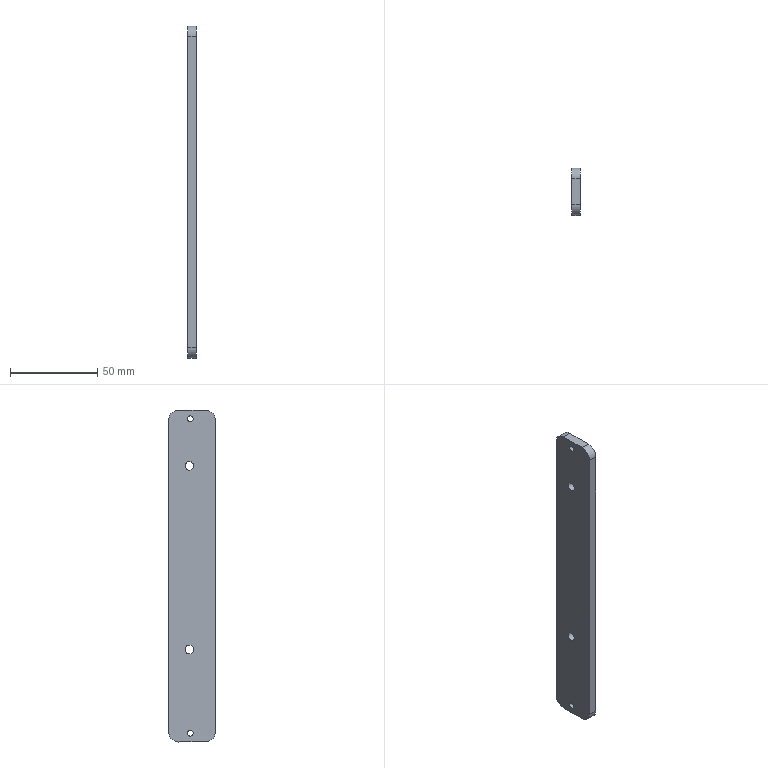Part | NX | 1 solid | 14 faces | box 5 x 27 x 190 mm | volume 25214 mm3 | cylinder 8 | plane 6 | commonest cylinder face diameters 12 x4 3.3 x2 5 x2
STEP:
#1=CARTESIAN_POINT('',(210.423,-113.198,-7.805));
#2=VERTEX_POINT('',#1);
#3=CARTESIAN_POINT('',(210.423,-113.198,170.195));
#4=VERTEX_POINT('',#3);
#5=CARTESIAN_POINT('',(210.423,-113.198,-13.805));
#6=DIRECTION('',(0.,0.,1.));
#7=VECTOR('',#6,1000.);
#8=LINE('',#5,#7);
#9=EDGE_CURVE('',#2,#4,#8,.T.);
#10=ORIENTED_EDGE('',*,*,#9,.F.);
#11=CARTESIAN_POINT('',(205.423,-113.198,-7.805));
#12=VERTEX_POINT('',#11);
#13=CARTESIAN_POINT('',(210.423,-113.198,-7.805));
#14=DIRECTION('',(-1.,0.,0.));
#15=VECTOR('',#14,1000.);
#16=LINE('',#13,#15);
#17=EDGE_CURVE('',#2,#12,#16,.T.);
#18=ORIENTED_EDGE('',*,*,#17,.T.);
#19=CARTESIAN_POINT('',(205.423,-113.198,170.195));
#20=VERTEX_POINT('',#19);
#21=CARTESIAN_POINT('',(205.423,-113.198,-13.805));
#22=DIRECTION('',(0.,0.,1.));
#23=VECTOR('',#22,1000.);
#24=LINE('',#21,#23);
#25=EDGE_CURVE('',#12,#20,#24,.T.);
#26=ORIENTED_EDGE('',*,*,#25,.T.);
#27=CARTESIAN_POINT('',(210.423,-113.198,170.195));
#28=DIRECTION('',(1.,0.,0.));
#29=VECTOR('',#28,1000.);
#30=LINE('',#27,#29);
#31=EDGE_CURVE('',#20,#4,#30,.T.);
#32=ORIENTED_EDGE('',*,*,#31,.T.);
#33=EDGE_LOOP('',(#10,#18,#26,#32));
#34=FACE_BOUND('',#33,.T.);
#35=CARTESIAN_POINT('',(210.423,-113.198,-13.805));
#36=DIRECTION('',(0.,-1.,0.));
#37=DIRECTION('',(-1.,0.,0.));
#38=AXIS2_PLACEMENT_3D('',#35,#36,#37);
#39=PLANE('',#38);
#40=ADVANCED_FACE('',(#34),#39,.F.);
#41=CARTESIAN_POINT('',(205.423,-119.198,176.195));
#42=VERTEX_POINT('',#41);
#43=CARTESIAN_POINT('',(205.423,-134.198,176.195));
#44=VERTEX_POINT('',#43);
#45=CARTESIAN_POINT('',(205.423,-140.198,176.195));
#46=DIRECTION('',(0.,-1.,0.));
#47=VECTOR('',#46,1000.);
#48=LINE('',#45,#47);
#49=EDGE_CURVE('',#42,#44,#48,.T.);
#50=ORIENTED_EDGE('',*,*,#49,.T.);
#51=CARTESIAN_POINT('',(210.423,-134.198,176.195));
#52=VERTEX_POINT('',#51);
#53=CARTESIAN_POINT('',(210.423,-134.198,176.195));
#54=DIRECTION('',(1.,0.,0.));
#55=VECTOR('',#54,1000.);
#56=LINE('',#53,#55);
#57=EDGE_CURVE('',#44,#52,#56,.T.);
#58=ORIENTED_EDGE('',*,*,#57,.T.);
#59=CARTESIAN_POINT('',(210.423,-119.198,176.195));
#60=VERTEX_POINT('',#59);
#61=CARTESIAN_POINT('',(210.423,-140.198,176.195));
#62=DIRECTION('',(0.,-1.,0.));
#63=VECTOR('',#62,1000.);
#64=LINE('',#61,#63);
#65=EDGE_CURVE('',#60,#52,#64,.T.);
#66=ORIENTED_EDGE('',*,*,#65,.F.);
#67=CARTESIAN_POINT('',(210.423,-119.198,176.195));
#68=DIRECTION('',(-1.,0.,0.));
#69=VECTOR('',#68,1000.);
#70=LINE('',#67,#69);
#71=EDGE_CURVE('',#60,#42,#70,.T.);
#72=ORIENTED_EDGE('',*,*,#71,.T.);
#73=EDGE_LOOP('',(#50,#58,#66,#72));
#74=FACE_BOUND('',#73,.T.);
#75=CARTESIAN_POINT('',(210.423,-140.198,176.195));
#76=DIRECTION('',(0.,0.,-1.));
#77=DIRECTION('',(0.,-1.,0.));
#78=AXIS2_PLACEMENT_3D('',#75,#76,#77);
#79=PLANE('',#78);
#80=ADVANCED_FACE('',(#74),#79,.F.);
#81=CARTESIAN_POINT('',(205.423,-140.198,170.195));
#82=VERTEX_POINT('',#81);
#83=CARTESIAN_POINT('',(205.423,-140.198,-7.805));
#84=VERTEX_POINT('',#83);
#85=CARTESIAN_POINT('',(205.423,-140.198,-13.805));
#86=DIRECTION('',(0.,0.,-1.));
#87=VECTOR('',#86,1000.);
#88=LINE('',#85,#87);
#89=EDGE_CURVE('',#82,#84,#88,.T.);
#90=ORIENTED_EDGE('',*,*,#89,.T.);
#91=CARTESIAN_POINT('',(210.423,-140.198,-7.805));
#92=VERTEX_POINT('',#91);
#93=CARTESIAN_POINT('',(210.423,-140.198,-7.805));
#94=DIRECTION('',(1.,0.,0.));
#95=VECTOR('',#94,1000.);
#96=LINE('',#93,#95);
#97=EDGE_CURVE('',#84,#92,#96,.T.);
#98=ORIENTED_EDGE('',*,*,#97,.T.);
#99=CARTESIAN_POINT('',(210.423,-140.198,170.195));
#100=VERTEX_POINT('',#99);
#101=CARTESIAN_POINT('',(210.423,-140.198,-13.805));
#102=DIRECTION('',(0.,0.,-1.));
#103=VECTOR('',#102,1000.);
#104=LINE('',#101,#103);
#105=EDGE_CURVE('',#100,#92,#104,.T.);
#106=ORIENTED_EDGE('',*,*,#105,.F.);
#107=CARTESIAN_POINT('',(210.423,-140.198,170.195));
#108=DIRECTION('',(-1.,0.,0.));
#109=VECTOR('',#108,1000.);
#110=LINE('',#107,#109);
#111=EDGE_CURVE('',#100,#82,#110,.T.);
#112=ORIENTED_EDGE('',*,*,#111,.T.);
#113=EDGE_LOOP('',(#90,#98,#106,#112));
#114=FACE_BOUND('',#113,.T.);
#115=CARTESIAN_POINT('',(210.423,-140.198,-13.805));
#116=DIRECTION('',(0.,1.,0.));
#117=DIRECTION('',(0.,0.,-1.));
#118=AXIS2_PLACEMENT_3D('',#115,#116,#117);
#119=PLANE('',#118);
#120=ADVANCED_FACE('',(#114),#119,.F.);
#121=CARTESIAN_POINT('',(205.423,-134.198,-13.805));
#122=VERTEX_POINT('',#121);
#123=CARTESIAN_POINT('',(205.423,-119.198,-13.805));
#124=VERTEX_POINT('',#123);
#125=CARTESIAN_POINT('',(205.423,-140.198,-13.805));
#126=DIRECTION('',(0.,1.,0.));
#127=VECTOR('',#126,1000.);
#128=LINE('',#125,#127);
#129=EDGE_CURVE('',#122,#124,#128,.T.);
#130=ORIENTED_EDGE('',*,*,#129,.T.);
#131=CARTESIAN_POINT('',(210.423,-119.198,-13.805));
#132=VERTEX_POINT('',#131);
#133=CARTESIAN_POINT('',(210.423,-119.198,-13.805));
#134=DIRECTION('',(1.,0.,0.));
#135=VECTOR('',#134,1000.);
#136=LINE('',#133,#135);
#137=EDGE_CURVE('',#124,#132,#136,.T.);
#138=ORIENTED_EDGE('',*,*,#137,.T.);
#139=CARTESIAN_POINT('',(210.423,-134.198,-13.805));
#140=VERTEX_POINT('',#139);
#141=CARTESIAN_POINT('',(210.423,-140.198,-13.805));
#142=DIRECTION('',(0.,1.,0.));
#143=VECTOR('',#142,1000.);
#144=LINE('',#141,#143);
#145=EDGE_CURVE('',#140,#132,#144,.T.);
#146=ORIENTED_EDGE('',*,*,#145,.F.);
#147=CARTESIAN_POINT('',(210.423,-134.198,-13.805));
#148=DIRECTION('',(-1.,0.,0.));
#149=VECTOR('',#148,1000.);
#150=LINE('',#147,#149);
#151=EDGE_CURVE('',#140,#122,#150,.T.);
#152=ORIENTED_EDGE('',*,*,#151,.T.);
#153=EDGE_LOOP('',(#130,#138,#146,#152));
#154=FACE_BOUND('',#153,.T.);
#155=CARTESIAN_POINT('',(210.423,-140.198,-13.805));
#156=DIRECTION('',(0.,0.,1.));
#157=DIRECTION('',(0.,-1.,0.));
#158=AXIS2_PLACEMENT_3D('',#155,#156,#157);
#159=PLANE('',#158);
#160=ADVANCED_FACE('',(#154),#159,.F.);
#161=CARTESIAN_POINT('',(210.423,-127.744,144.196));
#162=VERTEX_POINT('',#161);
#163=CARTESIAN_POINT('',(210.423,-125.244,144.196));
#164=DIRECTION('',(1.,0.,0.));
#165=DIRECTION('',(0.,-1.,0.));
#166=AXIS2_PLACEMENT_3D('',#163,#164,#165);
#167=CIRCLE('',#166,2.5);
#168=EDGE_CURVE('',#162,#162,#167,.T.);
#169=ORIENTED_EDGE('',*,*,#168,.F.);
#170=EDGE_LOOP('',(#169));
#171=FACE_BOUND('',#170,.T.);
#172=CARTESIAN_POINT('',(210.423,-127.744,39.152));
#173=VERTEX_POINT('',#172);
#174=CARTESIAN_POINT('',(210.423,-125.244,39.152));
#175=DIRECTION('',(1.,0.,0.));
#176=DIRECTION('',(0.,-1.,0.));
#177=AXIS2_PLACEMENT_3D('',#174,#175,#176);
#178=CIRCLE('',#177,2.5);
#179=EDGE_CURVE('',#173,#173,#178,.T.);
#180=ORIENTED_EDGE('',*,*,#179,.F.);
#181=EDGE_LOOP('',(#180));
#182=FACE_BOUND('',#181,.T.);
#183=CARTESIAN_POINT('',(210.423,-127.348,171.2));
#184=VERTEX_POINT('',#183);
#185=CARTESIAN_POINT('',(210.423,-125.698,171.2));
#186=DIRECTION('',(-1.,0.,0.));
#187=DIRECTION('',(0.,-1.,0.));
#188=AXIS2_PLACEMENT_3D('',#185,#186,#187);
#189=CIRCLE('',#188,1.65);
#190=EDGE_CURVE('',#184,#184,#189,.T.);
#191=ORIENTED_EDGE('',*,*,#190,.T.);
#192=EDGE_LOOP('',(#191));
#193=FACE_BOUND('',#192,.T.);
#194=CARTESIAN_POINT('',(210.423,-127.348,-8.8));
#195=VERTEX_POINT('',#194);
#196=CARTESIAN_POINT('',(210.423,-125.698,-8.8));
#197=DIRECTION('',(-1.,0.,0.));
#198=DIRECTION('',(0.,-1.,0.));
#199=AXIS2_PLACEMENT_3D('',#196,#197,#198);
#200=CIRCLE('',#199,1.65);
#201=EDGE_CURVE('',#195,#195,#200,.T.);
#202=ORIENTED_EDGE('',*,*,#201,.T.);
#203=EDGE_LOOP('',(#202));
#204=FACE_BOUND('',#203,.T.);
#205=ORIENTED_EDGE('',*,*,#145,.T.);
#206=CARTESIAN_POINT('',(210.423,-119.198,-7.805));
#207=DIRECTION('',(1.,0.,0.));
#208=DIRECTION('',(0.,-1.,0.));
#209=AXIS2_PLACEMENT_3D('',#206,#207,#208);
#210=CIRCLE('',#209,6.);
#211=EDGE_CURVE('',#132,#2,#210,.T.);
#212=ORIENTED_EDGE('',*,*,#211,.T.);
#213=ORIENTED_EDGE('',*,*,#9,.T.);
#214=CARTESIAN_POINT('',(210.423,-119.198,170.195));
#215=DIRECTION('',(1.,0.,0.));
#216=DIRECTION('',(0.,-1.,0.));
#217=AXIS2_PLACEMENT_3D('',#214,#215,#216);
#218=CIRCLE('',#217,6.);
#219=EDGE_CURVE('',#4,#60,#218,.T.);
#220=ORIENTED_EDGE('',*,*,#219,.T.);
#221=ORIENTED_EDGE('',*,*,#65,.T.);
#222=CARTESIAN_POINT('',(210.423,-134.198,170.195));
#223=DIRECTION('',(1.,0.,0.));
#224=DIRECTION('',(0.,-1.,0.));
#225=AXIS2_PLACEMENT_3D('',#222,#223,#224);
#226=CIRCLE('',#225,6.);
#227=EDGE_CURVE('',#52,#100,#226,.T.);
#228=ORIENTED_EDGE('',*,*,#227,.T.);
#229=ORIENTED_EDGE('',*,*,#105,.T.);
#230=CARTESIAN_POINT('',(210.423,-134.198,-7.805));
#231=DIRECTION('',(1.,0.,0.));
#232=DIRECTION('',(0.,-1.,0.));
#233=AXIS2_PLACEMENT_3D('',#230,#231,#232);
#234=CIRCLE('',#233,6.);
#235=EDGE_CURVE('',#92,#140,#234,.T.);
#236=ORIENTED_EDGE('',*,*,#235,.T.);
#237=EDGE_LOOP('',(#205,#212,#213,#220,#221,#228,#229,#236));
#238=FACE_BOUND('',#237,.T.);
#239=CARTESIAN_POINT('',(210.423,-126.698,81.195));
#240=DIRECTION('',(-1.,0.,0.));
#241=DIRECTION('',(0.,1.,0.));
#242=AXIS2_PLACEMENT_3D('',#239,#240,#241);
#243=PLANE('',#242);
#244=ADVANCED_FACE('',(#171,#182,#193,#204,#238),#243,.F.);
#245=CARTESIAN_POINT('',(205.423,-127.744,144.196));
#246=VERTEX_POINT('',#245);
#247=CARTESIAN_POINT('',(205.423,-125.244,144.196));
#248=DIRECTION('',(1.,0.,0.));
#249=DIRECTION('',(0.,-1.,0.));
#250=AXIS2_PLACEMENT_3D('',#247,#248,#249);
#251=CIRCLE('',#250,2.5);
#252=EDGE_CURVE('',#246,#246,#251,.T.);
#253=ORIENTED_EDGE('',*,*,#252,.T.);
#254=EDGE_LOOP('',(#253));
#255=FACE_BOUND('',#254,.T.);
#256=CARTESIAN_POINT('',(205.423,-127.744,39.152));
#257=VERTEX_POINT('',#256);
#258=CARTESIAN_POINT('',(205.423,-125.244,39.152));
#259=DIRECTION('',(1.,0.,0.));
#260=DIRECTION('',(0.,-1.,0.));
#261=AXIS2_PLACEMENT_3D('',#258,#259,#260);
#262=CIRCLE('',#261,2.5);
#263=EDGE_CURVE('',#257,#257,#262,.T.);
#264=ORIENTED_EDGE('',*,*,#263,.T.);
#265=EDGE_LOOP('',(#264));
#266=FACE_BOUND('',#265,.T.);
#267=CARTESIAN_POINT('',(205.423,-127.348,171.2));
#268=VERTEX_POINT('',#267);
#269=CARTESIAN_POINT('',(205.423,-125.698,171.2));
#270=DIRECTION('',(-1.,0.,0.));
#271=DIRECTION('',(0.,-1.,0.));
#272=AXIS2_PLACEMENT_3D('',#269,#270,#271);
#273=CIRCLE('',#272,1.65);
#274=EDGE_CURVE('',#268,#268,#273,.T.);
#275=ORIENTED_EDGE('',*,*,#274,.F.);
#276=EDGE_LOOP('',(#275));
#277=FACE_BOUND('',#276,.T.);
#278=CARTESIAN_POINT('',(205.423,-127.348,-8.8));
#279=VERTEX_POINT('',#278);
#280=CARTESIAN_POINT('',(205.423,-125.698,-8.8));
#281=DIRECTION('',(-1.,0.,0.));
#282=DIRECTION('',(0.,-1.,0.));
#283=AXIS2_PLACEMENT_3D('',#280,#281,#282);
#284=CIRCLE('',#283,1.65);
#285=EDGE_CURVE('',#279,#279,#284,.T.);
#286=ORIENTED_EDGE('',*,*,#285,.F.);
#287=EDGE_LOOP('',(#286));
#288=FACE_BOUND('',#287,.T.);
#289=ORIENTED_EDGE('',*,*,#25,.F.);
#290=CARTESIAN_POINT('',(205.423,-119.198,-7.805));
#291=DIRECTION('',(-1.,0.,0.));
#292=DIRECTION('',(0.,-1.,0.));
#293=AXIS2_PLACEMENT_3D('',#290,#291,#292);
#294=CIRCLE('',#293,6.);
#295=EDGE_CURVE('',#12,#124,#294,.T.);
#296=ORIENTED_EDGE('',*,*,#295,.T.);
#297=ORIENTED_EDGE('',*,*,#129,.F.);
#298=CARTESIAN_POINT('',(205.423,-134.198,-7.805));
#299=DIRECTION('',(-1.,0.,0.));
#300=DIRECTION('',(0.,-1.,0.));
#301=AXIS2_PLACEMENT_3D('',#298,#299,#300);
#302=CIRCLE('',#301,6.);
#303=EDGE_CURVE('',#122,#84,#302,.T.);
#304=ORIENTED_EDGE('',*,*,#303,.T.);
#305=ORIENTED_EDGE('',*,*,#89,.F.);
#306=CARTESIAN_POINT('',(205.423,-134.198,170.195));
#307=DIRECTION('',(-1.,0.,0.));
#308=DIRECTION('',(0.,-1.,0.));
#309=AXIS2_PLACEMENT_3D('',#306,#307,#308);
#310=CIRCLE('',#309,6.);
#311=EDGE_CURVE('',#82,#44,#310,.T.);
#312=ORIENTED_EDGE('',*,*,#311,.T.);
#313=ORIENTED_EDGE('',*,*,#49,.F.);
#314=CARTESIAN_POINT('',(205.423,-119.198,170.195));
#315=DIRECTION('',(-1.,0.,0.));
#316=DIRECTION('',(0.,-1.,0.));
#317=AXIS2_PLACEMENT_3D('',#314,#315,#316);
#318=CIRCLE('',#317,6.);
#319=EDGE_CURVE('',#42,#20,#318,.T.);
#320=ORIENTED_EDGE('',*,*,#319,.T.);
#321=EDGE_LOOP('',(#289,#296,#297,#304,#305,#312,#313,#320));
#322=FACE_BOUND('',#321,.T.);
#323=CARTESIAN_POINT('',(205.423,-126.698,81.195));
#324=DIRECTION('',(-1.,0.,0.));
#325=DIRECTION('',(0.,1.,0.));
#326=AXIS2_PLACEMENT_3D('',#323,#324,#325);
#327=PLANE('',#326);
#328=ADVANCED_FACE('',(#255,#266,#277,#288,#322),#327,.T.);
#329=ORIENTED_EDGE('',*,*,#211,.F.);
#330=ORIENTED_EDGE('',*,*,#137,.F.);
#331=ORIENTED_EDGE('',*,*,#295,.F.);
#332=ORIENTED_EDGE('',*,*,#17,.F.);
#333=EDGE_LOOP('',(#329,#330,#331,#332));
#334=FACE_BOUND('',#333,.T.);
#335=CARTESIAN_POINT('',(210.423,-119.198,-7.805));
#336=DIRECTION('',(-1.,0.,0.));
#337=DIRECTION('',(0.,-1.,0.));
#338=AXIS2_PLACEMENT_3D('',#335,#336,#337);
#339=CYLINDRICAL_SURFACE('',#338,6.);
#340=ADVANCED_FACE('',(#334),#339,.T.);
#341=ORIENTED_EDGE('',*,*,#235,.F.);
#342=ORIENTED_EDGE('',*,*,#97,.F.);
#343=ORIENTED_EDGE('',*,*,#303,.F.);
#344=ORIENTED_EDGE('',*,*,#151,.F.);
#345=EDGE_LOOP('',(#341,#342,#343,#344));
#346=FACE_BOUND('',#345,.T.);
#347=CARTESIAN_POINT('',(210.423,-134.198,-7.805));
#348=DIRECTION('',(-1.,0.,0.));
#349=DIRECTION('',(0.,-1.,0.));
#350=AXIS2_PLACEMENT_3D('',#347,#348,#349);
#351=CYLINDRICAL_SURFACE('',#350,6.);
#352=ADVANCED_FACE('',(#346),#351,.T.);
#353=ORIENTED_EDGE('',*,*,#227,.F.);
#354=ORIENTED_EDGE('',*,*,#57,.F.);
#355=ORIENTED_EDGE('',*,*,#311,.F.);
#356=ORIENTED_EDGE('',*,*,#111,.F.);
#357=EDGE_LOOP('',(#353,#354,#355,#356));
#358=FACE_BOUND('',#357,.T.);
#359=CARTESIAN_POINT('',(210.423,-134.198,170.195));
#360=DIRECTION('',(-1.,0.,0.));
#361=DIRECTION('',(0.,-1.,0.));
#362=AXIS2_PLACEMENT_3D('',#359,#360,#361);
#363=CYLINDRICAL_SURFACE('',#362,6.);
#364=ADVANCED_FACE('',(#358),#363,.T.);
#365=ORIENTED_EDGE('',*,*,#219,.F.);
#366=ORIENTED_EDGE('',*,*,#31,.F.);
#367=ORIENTED_EDGE('',*,*,#319,.F.);
#368=ORIENTED_EDGE('',*,*,#71,.F.);
#369=EDGE_LOOP('',(#365,#366,#367,#368));
#370=FACE_BOUND('',#369,.T.);
#371=CARTESIAN_POINT('',(210.423,-119.198,170.195));
#372=DIRECTION('',(-1.,0.,0.));
#373=DIRECTION('',(0.,-1.,0.));
#374=AXIS2_PLACEMENT_3D('',#371,#372,#373);
#375=CYLINDRICAL_SURFACE('',#374,6.);
#376=ADVANCED_FACE('',(#370),#375,.T.);
#377=ORIENTED_EDGE('',*,*,#252,.F.);
#378=EDGE_LOOP('',(#377));
#379=FACE_BOUND('',#378,.T.);
#380=ORIENTED_EDGE('',*,*,#168,.T.);
#381=EDGE_LOOP('',(#380));
#382=FACE_BOUND('',#381,.T.);
#383=CARTESIAN_POINT('',(215.373,-125.244,144.196));
#384=DIRECTION('',(1.,0.,0.));
#385=DIRECTION('',(0.,1.,0.));
#386=AXIS2_PLACEMENT_3D('',#383,#384,#385);
#387=CYLINDRICAL_SURFACE('',#386,2.5);
#388=ADVANCED_FACE('',(#379,#382),#387,.F.);
#389=ORIENTED_EDGE('',*,*,#263,.F.);
#390=EDGE_LOOP('',(#389));
#391=FACE_BOUND('',#390,.T.);
#392=ORIENTED_EDGE('',*,*,#179,.T.);
#393=EDGE_LOOP('',(#392));
#394=FACE_BOUND('',#393,.T.);
#395=CARTESIAN_POINT('',(215.373,-125.244,39.152));
#396=DIRECTION('',(1.,0.,0.));
#397=DIRECTION('',(0.,1.,0.));
#398=AXIS2_PLACEMENT_3D('',#395,#396,#397);
#399=CYLINDRICAL_SURFACE('',#398,2.5);
#400=ADVANCED_FACE('',(#391,#394),#399,.F.);
#401=ORIENTED_EDGE('',*,*,#274,.T.);
#402=EDGE_LOOP('',(#401));
#403=FACE_BOUND('',#402,.T.);
#404=ORIENTED_EDGE('',*,*,#190,.F.);
#405=EDGE_LOOP('',(#404));
#406=FACE_BOUND('',#405,.T.);
#407=CARTESIAN_POINT('',(200.723,-125.698,171.2));
#408=DIRECTION('',(-1.,0.,0.));
#409=DIRECTION('',(0.,-1.,0.));
#410=AXIS2_PLACEMENT_3D('',#407,#408,#409);
#411=CYLINDRICAL_SURFACE('',#410,1.65);
#412=ADVANCED_FACE('',(#403,#406),#411,.F.);
#413=ORIENTED_EDGE('',*,*,#285,.T.);
#414=EDGE_LOOP('',(#413));
#415=FACE_BOUND('',#414,.T.);
#416=ORIENTED_EDGE('',*,*,#201,.F.);
#417=EDGE_LOOP('',(#416));
#418=FACE_BOUND('',#417,.T.);
#419=CARTESIAN_POINT('',(200.723,-125.698,-8.8));
#420=DIRECTION('',(-1.,0.,0.));
#421=DIRECTION('',(0.,-1.,0.));
#422=AXIS2_PLACEMENT_3D('',#419,#420,#421);
#423=CYLINDRICAL_SURFACE('',#422,1.65);
#424=ADVANCED_FACE('',(#415,#418),#423,.F.);
#425=CLOSED_SHELL('',(#40,#80,#120,#160,#244,#328,#340,#352,#364,#376,#388,#400,#412,#424));
#426=MANIFOLD_SOLID_BREP('',#425);
#427=(LENGTH_UNIT()NAMED_UNIT(*)SI_UNIT(.MILLI.,.METRE.));
#428=UNCERTAINTY_MEASURE_WITH_UNIT(LENGTH_MEASURE(0.00001),#427,'','');
#429=(NAMED_UNIT(*)PLANE_ANGLE_UNIT()SI_UNIT($,.RADIAN.));
#430=(NAMED_UNIT(*)SI_UNIT($,.STERADIAN.)SOLID_ANGLE_UNIT());
#431=(GEOMETRIC_REPRESENTATION_CONTEXT(3)GLOBAL_UNCERTAINTY_ASSIGNED_CONTEXT((#428))GLOBAL_UNIT_ASSIGNED_CONTEXT((#427,#429,#430))REPRESENTATION_CONTEXT('',''));
#432=ADVANCED_BREP_SHAPE_REPRESENTATION('',(#426),#431);